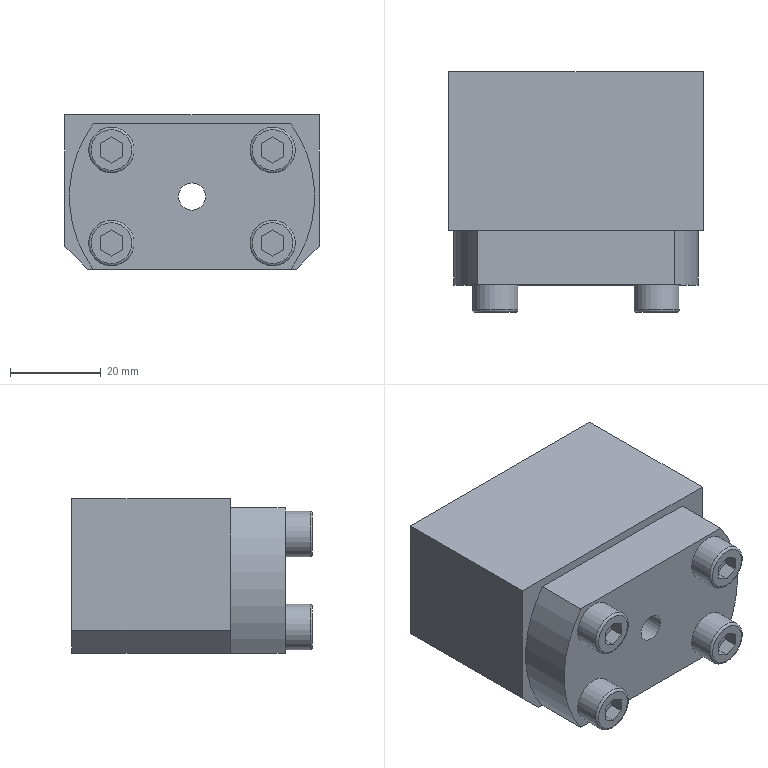Part | NX | features BREP 8, DATUM_CSYS 7, SKETCH 6, EXTRUDE 5, META 4, CHAMFER 1 | 5 solids | 107 faces | box 56 x 53 x 34 mm | volume 80707 mm3 | plane 70 | cylinder 25 | cone 8 | torus 4 | commonest cylinder face diameters 6 x9 5 x4 5.7 x4 10 x4 54 x2 30 x1